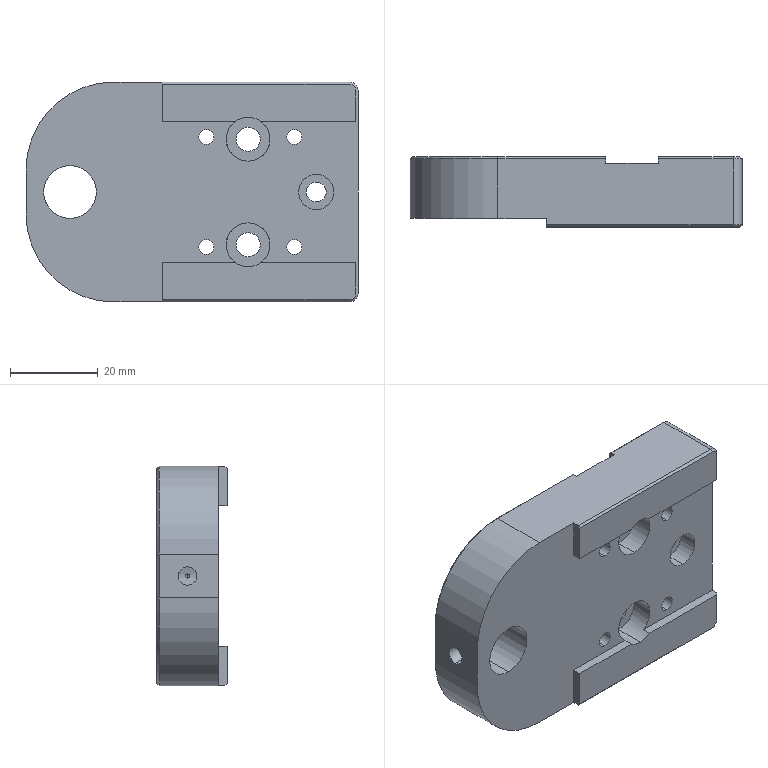Part | STEP file | ND25021-01-JDKM-26-TL | 1 solid | 87 faces | box 75.5 x 16 x 50 mm | volume 46652 mm3 | cylinder 40 | plane 35 | cone 12 | commonest cylinder face diameters 3.4 x8 6 x8 4.2 x6 5.5 x4 10 x4 4 x2